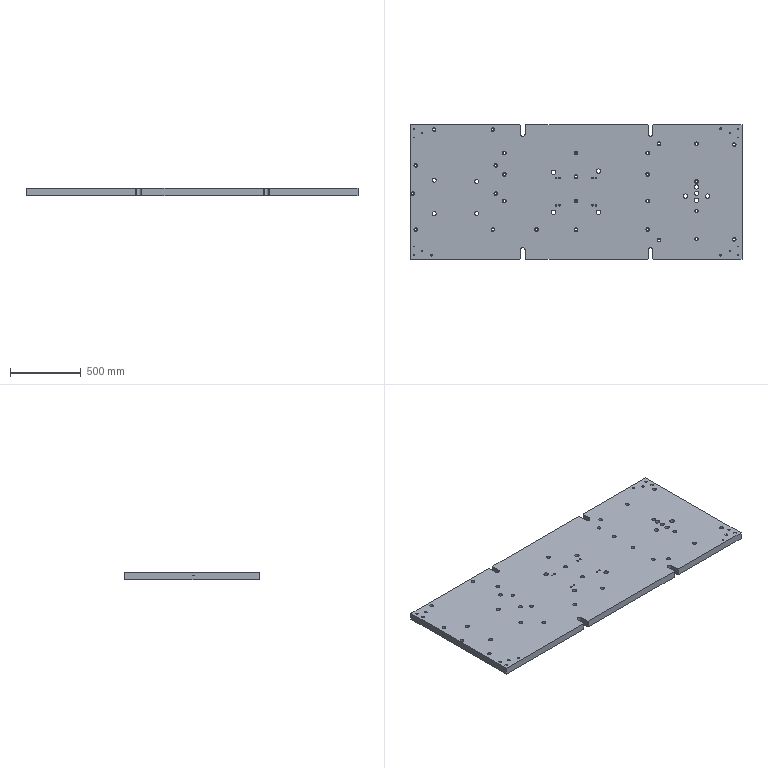Part | NX | features solid 2 | 1 solid | 226 faces | box 2340 x 950 x 50 mm | volume 109376317 mm3 | cylinder 108 | cone 56 | plane 54 | spline 8 | commonest cylinder face diameters 18.007 x28 26.008 x28 6.8 x16 21 x12 31 x9 11 x8